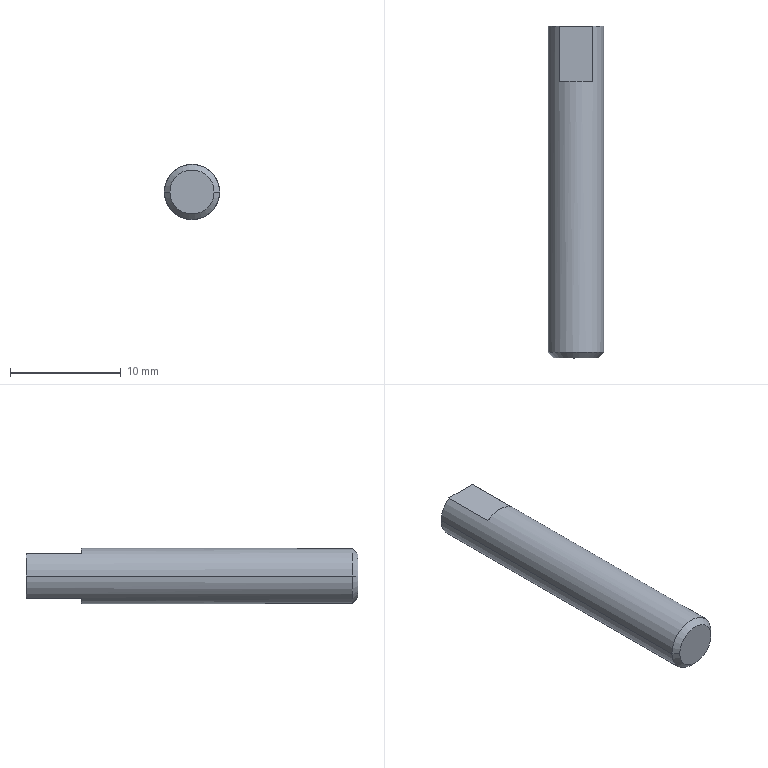Part | STEP file | BU-C08b-2 | 1 solid | 10 faces | box 5 x 30 x 5 mm | volume 576.997 mm3 | plane 6 | cone 2 | cylinder 2 | commonest cylinder face diameters 5 x2
STEP:
#1=CARTESIAN_POINT('',(0.,0.,0.));
#2=DIRECTION('',(0.,0.,1.));
#3=DIRECTION('',(1.,0.,0.));
#4=AXIS2_PLACEMENT_3D('',#1,#2,#3);
#5=CARTESIAN_POINT('',(2.,0.,0.));
#6=VERTEX_POINT('',#5);
#7=CARTESIAN_POINT('',(-2.,0.,0.));
#8=VERTEX_POINT('',#7);
#9=CARTESIAN_POINT('',(0.,0.,0.));
#10=DIRECTION('',(0.,-1.,0.));
#11=DIRECTION('',(1.,0.,0.));
#12=AXIS2_PLACEMENT_3D('',#9,#10,#11);
#13=CIRCLE('',#12,2.);
#14=CARTESIAN_POINT('',(0.,0.,0.));
#15=DIRECTION('',(0.,1.,0.));
#16=DIRECTION('',(-1.,0.,0.));
#17=AXIS2_PLACEMENT_3D('',#14,#15,#16);
#18=CONICAL_SURFACE('',#17,2.,0.7854);
#19=CARTESIAN_POINT('',(3.142,0.));
#20=DIRECTION('',(-1.,0.));
#21=VECTOR('',#20,1.);
#22=LINE('',#19,#21);
#23=(GEOMETRIC_REPRESENTATION_CONTEXT(2)PARAMETRIC_REPRESENTATION_CONTEXT()REPRESENTATION_CONTEXT('',''));
#24=DEFINITIONAL_REPRESENTATION('',(#22),#23);
#25=PCURVE('',#18,#24);
#26=CARTESIAN_POINT('',(0.,0.,0.));
#27=DIRECTION('',(0.,-1.,0.));
#28=DIRECTION('',(1.,0.,0.));
#29=AXIS2_PLACEMENT_3D('',#26,#27,#28);
#30=PLANE('',#29);
#31=CARTESIAN_POINT('',(0.,0.));
#32=DIRECTION('',(1.,0.));
#33=AXIS2_PLACEMENT_2D('',#31,#32);
#34=CIRCLE('',#33,2.);
#35=(GEOMETRIC_REPRESENTATION_CONTEXT(2)PARAMETRIC_REPRESENTATION_CONTEXT()REPRESENTATION_CONTEXT('',''));
#36=DEFINITIONAL_REPRESENTATION('',(#34),#35);
#37=PCURVE('',#30,#36);
#38=SURFACE_CURVE('',#13,(#25,#37),.PCURVE_S1.);
#39=EDGE_CURVE('',#6,#8,#38,.T.);
#40=ORIENTED_EDGE('',*,*,#39,.F.);
#41=CARTESIAN_POINT('',(2.5,0.5,0.));
#42=VERTEX_POINT('',#41);
#43=CARTESIAN_POINT('',(2.,0.,0.));
#44=DIRECTION('',(0.7071,0.7071,0.));
#45=VECTOR('',#44,1.);
#46=LINE('',#43,#45);
#47=CARTESIAN_POINT('',(3.142,0.));
#48=DIRECTION('',(0.,1.));
#49=VECTOR('',#48,1.);
#50=LINE('',#47,#49);
#51=(GEOMETRIC_REPRESENTATION_CONTEXT(2)PARAMETRIC_REPRESENTATION_CONTEXT()REPRESENTATION_CONTEXT('',''));
#52=DEFINITIONAL_REPRESENTATION('',(#50),#51);
#53=PCURVE('',#18,#52);
#54=CARTESIAN_POINT('',(0.,0.,0.));
#55=DIRECTION('',(0.,1.,0.));
#56=DIRECTION('',(-1.,0.,0.));
#57=AXIS2_PLACEMENT_3D('',#54,#55,#56);
#58=CONICAL_SURFACE('',#57,2.,0.7854);
#59=CARTESIAN_POINT('',(3.142,0.));
#60=DIRECTION('',(0.,1.));
#61=VECTOR('',#60,1.);
#62=LINE('',#59,#61);
#63=(GEOMETRIC_REPRESENTATION_CONTEXT(2)PARAMETRIC_REPRESENTATION_CONTEXT()REPRESENTATION_CONTEXT('',''));
#64=DEFINITIONAL_REPRESENTATION('',(#62),#63);
#65=PCURVE('',#58,#64);
#66=SURFACE_CURVE('',#46,(#53,#65),.PCURVE_S1.);
#67=EDGE_CURVE('',#6,#42,#66,.T.);
#68=ORIENTED_EDGE('',*,*,#67,.T.);
#69=CARTESIAN_POINT('',(-2.5,0.5,0.));
#70=VERTEX_POINT('',#69);
#71=CARTESIAN_POINT('',(0.,0.5,0.));
#72=DIRECTION('',(0.,1.,0.));
#73=DIRECTION('',(1.,0.,0.));
#74=AXIS2_PLACEMENT_3D('',#71,#72,#73);
#75=CIRCLE('',#74,2.5);
#76=CARTESIAN_POINT('',(-3.142,0.5));
#77=DIRECTION('',(1.,0.));
#78=VECTOR('',#77,1.);
#79=LINE('',#76,#78);
#80=(GEOMETRIC_REPRESENTATION_CONTEXT(2)PARAMETRIC_REPRESENTATION_CONTEXT()REPRESENTATION_CONTEXT('',''));
#81=DEFINITIONAL_REPRESENTATION('',(#79),#80);
#82=PCURVE('',#18,#81);
#83=CARTESIAN_POINT('',(0.,-1000.,0.));
#84=DIRECTION('',(0.,-1.,0.));
#85=DIRECTION('',(1.,0.,0.));
#86=AXIS2_PLACEMENT_3D('',#83,#84,#85);
#87=CYLINDRICAL_SURFACE('',#86,2.5);
#88=CARTESIAN_POINT('',(6.283,-1000.5));
#89=DIRECTION('',(-1.,0.));
#90=VECTOR('',#89,1.);
#91=LINE('',#88,#90);
#92=(GEOMETRIC_REPRESENTATION_CONTEXT(2)PARAMETRIC_REPRESENTATION_CONTEXT()REPRESENTATION_CONTEXT('',''));
#93=DEFINITIONAL_REPRESENTATION('',(#91),#92);
#94=PCURVE('',#87,#93);
#95=SURFACE_CURVE('',#75,(#82,#94),.PCURVE_S1.);
#96=EDGE_CURVE('',#70,#42,#95,.T.);
#97=ORIENTED_EDGE('',*,*,#96,.F.);
#98=CARTESIAN_POINT('',(-2.,0.,0.));
#99=DIRECTION('',(-0.7071,0.7071,0.));
#100=VECTOR('',#99,1.);
#101=LINE('',#98,#100);
#102=CARTESIAN_POINT('',(0.,0.));
#103=DIRECTION('',(0.,1.));
#104=VECTOR('',#103,1.);
#105=LINE('',#102,#104);
#106=(GEOMETRIC_REPRESENTATION_CONTEXT(2)PARAMETRIC_REPRESENTATION_CONTEXT()REPRESENTATION_CONTEXT('',''));
#107=DEFINITIONAL_REPRESENTATION('',(#105),#106);
#108=PCURVE('',#18,#107);
#109=CARTESIAN_POINT('',(6.283,0.));
#110=DIRECTION('',(0.,1.));
#111=VECTOR('',#110,1.);
#112=LINE('',#109,#111);
#113=(GEOMETRIC_REPRESENTATION_CONTEXT(2)PARAMETRIC_REPRESENTATION_CONTEXT()REPRESENTATION_CONTEXT('',''));
#114=DEFINITIONAL_REPRESENTATION('',(#112),#113);
#115=PCURVE('',#58,#114);
#116=SURFACE_CURVE('',#101,(#108,#115),.PCURVE_S1.);
#117=EDGE_CURVE('',#8,#70,#116,.T.);
#118=ORIENTED_EDGE('',*,*,#117,.F.);
#119=EDGE_LOOP('',(#40,#68,#97,#118));
#120=FACE_BOUND('',#119,.T.);
#121=ADVANCED_FACE('',(#120),#18,.T.);
#122=CARTESIAN_POINT('',(-1.5,30.,2.));
#123=VERTEX_POINT('',#122);
#124=CARTESIAN_POINT('',(-2.5,30.,0.));
#125=VERTEX_POINT('',#124);
#126=CARTESIAN_POINT('',(0.,30.,0.));
#127=DIRECTION('',(0.,-1.,0.));
#128=DIRECTION('',(1.,0.,0.));
#129=AXIS2_PLACEMENT_3D('',#126,#127,#128);
#130=CIRCLE('',#129,2.5);
#131=CARTESIAN_POINT('',(0.,-1030.));
#132=DIRECTION('',(1.,0.));
#133=VECTOR('',#132,1.);
#134=LINE('',#131,#133);
#135=(GEOMETRIC_REPRESENTATION_CONTEXT(2)PARAMETRIC_REPRESENTATION_CONTEXT()REPRESENTATION_CONTEXT('',''));
#136=DEFINITIONAL_REPRESENTATION('',(#134),#135);
#137=PCURVE('',#87,#136);
#138=CARTESIAN_POINT('',(0.,30.,0.));
#139=DIRECTION('',(0.,1.,0.));
#140=DIRECTION('',(-1.,0.,0.));
#141=AXIS2_PLACEMENT_3D('',#138,#139,#140);
#142=PLANE('',#141);
#143=CARTESIAN_POINT('',(-2.5,0.));
#144=CARTESIAN_POINT('',(-2.5,4.33));
#145=CARTESIAN_POINT('',(1.25,2.165));
#146=CARTESIAN_POINT('',(5.,0.));
#147=CARTESIAN_POINT('',(1.25,-2.165));
#148=CARTESIAN_POINT('',(-2.5,-4.33));
#149=CARTESIAN_POINT('',(-2.5,0.));
#150=(BOUNDED_CURVE()B_SPLINE_CURVE(2,(#143,#144,#145,#146,#147,#148,#149),.UNSPECIFIED.,.T.,.F.)B_SPLINE_CURVE_WITH_KNOTS((1,2,2,2,2,1),(-2.094,0.,2.094,4.189,6.283,8.378),.UNSPECIFIED.)CURVE()GEOMETRIC_REPRESENTATION_ITEM()RATIONAL_B_SPLINE_CURVE((1.,0.5,1.,0.5,1.,0.5,1.))REPRESENTATION_ITEM(''));
#151=(GEOMETRIC_REPRESENTATION_CONTEXT(2)PARAMETRIC_REPRESENTATION_CONTEXT()REPRESENTATION_CONTEXT('',''));
#152=DEFINITIONAL_REPRESENTATION('',(#150),#151);
#153=PCURVE('',#142,#152);
#154=SURFACE_CURVE('',#130,(#137,#153),.PCURVE_S1.);
#155=EDGE_CURVE('',#123,#125,#154,.T.);
#156=ORIENTED_EDGE('',*,*,#155,.T.);
#157=CARTESIAN_POINT('',(-2.5,-1000.,0.));
#158=DIRECTION('',(0.,-1.,0.));
#159=VECTOR('',#158,1.);
#160=LINE('',#157,#159);
#161=CARTESIAN_POINT('',(3.142,0.));
#162=DIRECTION('',(0.,1.));
#163=VECTOR('',#162,1.);
#164=LINE('',#161,#163);
#165=(GEOMETRIC_REPRESENTATION_CONTEXT(2)PARAMETRIC_REPRESENTATION_CONTEXT()REPRESENTATION_CONTEXT('',''));
#166=DEFINITIONAL_REPRESENTATION('',(#164),#165);
#167=PCURVE('',#87,#166);
#168=CARTESIAN_POINT('',(0.,-1000.,0.));
#169=DIRECTION('',(0.,-1.,0.));
#170=DIRECTION('',(1.,0.,0.));
#171=AXIS2_PLACEMENT_3D('',#168,#169,#170);
#172=CYLINDRICAL_SURFACE('',#171,2.5);
#173=CARTESIAN_POINT('',(3.142,0.));
#174=DIRECTION('',(0.,1.));
#175=VECTOR('',#174,1.);
#176=LINE('',#173,#175);
#177=(GEOMETRIC_REPRESENTATION_CONTEXT(2)PARAMETRIC_REPRESENTATION_CONTEXT()REPRESENTATION_CONTEXT('',''));
#178=DEFINITIONAL_REPRESENTATION('',(#176),#177);
#179=PCURVE('',#172,#178);
#180=SURFACE_CURVE('',#160,(#167,#179),.PCURVE_S1.);
#181=EDGE_CURVE('',#125,#70,#180,.T.);
#182=ORIENTED_EDGE('',*,*,#181,.T.);
#183=ORIENTED_EDGE('',*,*,#96,.T.);
#184=CARTESIAN_POINT('',(2.5,30.,0.));
#185=VERTEX_POINT('',#184);
#186=CARTESIAN_POINT('',(2.5,-1000.,0.));
#187=DIRECTION('',(0.,-1.,0.));
#188=VECTOR('',#187,1.);
#189=LINE('',#186,#188);
#190=CARTESIAN_POINT('',(0.,0.));
#191=DIRECTION('',(0.,1.));
#192=VECTOR('',#191,1.);
#193=LINE('',#190,#192);
#194=(GEOMETRIC_REPRESENTATION_CONTEXT(2)PARAMETRIC_REPRESENTATION_CONTEXT()REPRESENTATION_CONTEXT('',''));
#195=DEFINITIONAL_REPRESENTATION('',(#193),#194);
#196=PCURVE('',#87,#195);
#197=CARTESIAN_POINT('',(6.283,0.));
#198=DIRECTION('',(0.,1.));
#199=VECTOR('',#198,1.);
#200=LINE('',#197,#199);
#201=(GEOMETRIC_REPRESENTATION_CONTEXT(2)PARAMETRIC_REPRESENTATION_CONTEXT()REPRESENTATION_CONTEXT('',''));
#202=DEFINITIONAL_REPRESENTATION('',(#200),#201);
#203=PCURVE('',#172,#202);
#204=SURFACE_CURVE('',#189,(#196,#203),.PCURVE_S1.);
#205=EDGE_CURVE('',#185,#42,#204,.T.);
#206=ORIENTED_EDGE('',*,*,#205,.F.);
#207=CARTESIAN_POINT('',(1.5,30.,2.));
#208=VERTEX_POINT('',#207);
#209=CARTESIAN_POINT('',(0.,30.,0.));
#210=DIRECTION('',(0.,-1.,0.));
#211=DIRECTION('',(1.,0.,0.));
#212=AXIS2_PLACEMENT_3D('',#209,#210,#211);
#213=CIRCLE('',#212,2.5);
#214=CARTESIAN_POINT('',(0.,-1030.));
#215=DIRECTION('',(1.,0.));
#216=VECTOR('',#215,1.);
#217=LINE('',#214,#216);
#218=(GEOMETRIC_REPRESENTATION_CONTEXT(2)PARAMETRIC_REPRESENTATION_CONTEXT()REPRESENTATION_CONTEXT('',''));
#219=DEFINITIONAL_REPRESENTATION('',(#217),#218);
#220=PCURVE('',#87,#219);
#221=CARTESIAN_POINT('',(-2.5,0.));
#222=CARTESIAN_POINT('',(-2.5,4.33));
#223=CARTESIAN_POINT('',(1.25,2.165));
#224=CARTESIAN_POINT('',(5.,0.));
#225=CARTESIAN_POINT('',(1.25,-2.165));
#226=CARTESIAN_POINT('',(-2.5,-4.33));
#227=CARTESIAN_POINT('',(-2.5,0.));
#228=(BOUNDED_CURVE()B_SPLINE_CURVE(2,(#221,#222,#223,#224,#225,#226,#227),.UNSPECIFIED.,.T.,.F.)B_SPLINE_CURVE_WITH_KNOTS((1,2,2,2,2,1),(-2.094,0.,2.094,4.189,6.283,8.378),.UNSPECIFIED.)CURVE()GEOMETRIC_REPRESENTATION_ITEM()RATIONAL_B_SPLINE_CURVE((1.,0.5,1.,0.5,1.,0.5,1.))REPRESENTATION_ITEM(''));
#229=(GEOMETRIC_REPRESENTATION_CONTEXT(2)PARAMETRIC_REPRESENTATION_CONTEXT()REPRESENTATION_CONTEXT('',''));
#230=DEFINITIONAL_REPRESENTATION('',(#228),#229);
#231=PCURVE('',#142,#230);
#232=SURFACE_CURVE('',#213,(#220,#231),.PCURVE_S1.);
#233=EDGE_CURVE('',#185,#208,#232,.T.);
#234=ORIENTED_EDGE('',*,*,#233,.T.);
#235=CARTESIAN_POINT('',(1.5,25.,2.));
#236=VERTEX_POINT('',#235);
#237=CARTESIAN_POINT('',(1.5,25.,2.));
#238=DIRECTION('',(0.,1.,0.));
#239=VECTOR('',#238,1.);
#240=LINE('',#237,#239);
#241=CARTESIAN_POINT('',(0.9273,-1025.));
#242=DIRECTION('',(0.,-1.));
#243=VECTOR('',#242,1.);
#244=LINE('',#241,#243);
#245=(GEOMETRIC_REPRESENTATION_CONTEXT(2)PARAMETRIC_REPRESENTATION_CONTEXT()REPRESENTATION_CONTEXT('',''));
#246=DEFINITIONAL_REPRESENTATION('',(#244),#245);
#247=PCURVE('',#87,#246);
#248=CARTESIAN_POINT('',(-1.5,25.,2.));
#249=DIRECTION('',(0.,0.,-1.));
#250=DIRECTION('',(-1.,0.,0.));
#251=AXIS2_PLACEMENT_3D('',#248,#249,#250);
#252=PLANE('',#251);
#253=CARTESIAN_POINT('',(-3.,0.));
#254=DIRECTION('',(0.,1.));
#255=VECTOR('',#254,1.);
#256=LINE('',#253,#255);
#257=(GEOMETRIC_REPRESENTATION_CONTEXT(2)PARAMETRIC_REPRESENTATION_CONTEXT()REPRESENTATION_CONTEXT('',''));
#258=DEFINITIONAL_REPRESENTATION('',(#256),#257);
#259=PCURVE('',#252,#258);
#260=SURFACE_CURVE('',#240,(#247,#259),.PCURVE_S1.);
#261=EDGE_CURVE('',#236,#208,#260,.T.);
#262=ORIENTED_EDGE('',*,*,#261,.F.);
#263=CARTESIAN_POINT('',(-1.5,25.,2.));
#264=VERTEX_POINT('',#263);
#265=CARTESIAN_POINT('',(0.,25.,0.));
#266=DIRECTION('',(0.,1.,0.));
#267=DIRECTION('',(-1.,0.,0.));
#268=AXIS2_PLACEMENT_3D('',#265,#266,#267);
#269=CIRCLE('',#268,2.5);
#270=CARTESIAN_POINT('',(3.142,-1025.));
#271=DIRECTION('',(-1.,0.));
#272=VECTOR('',#271,1.);
#273=LINE('',#270,#272);
#274=(GEOMETRIC_REPRESENTATION_CONTEXT(2)PARAMETRIC_REPRESENTATION_CONTEXT()REPRESENTATION_CONTEXT('',''));
#275=DEFINITIONAL_REPRESENTATION('',(#273),#274);
#276=PCURVE('',#87,#275);
#277=CARTESIAN_POINT('',(0.,25.,0.));
#278=DIRECTION('',(0.,1.,0.));
#279=DIRECTION('',(-1.,0.,0.));
#280=AXIS2_PLACEMENT_3D('',#277,#278,#279);
#281=PLANE('',#280);
#282=CARTESIAN_POINT('',(0.,0.));
#283=DIRECTION('',(1.,0.));
#284=AXIS2_PLACEMENT_2D('',#282,#283);
#285=CIRCLE('',#284,2.5);
#286=(GEOMETRIC_REPRESENTATION_CONTEXT(2)PARAMETRIC_REPRESENTATION_CONTEXT()REPRESENTATION_CONTEXT('',''));
#287=DEFINITIONAL_REPRESENTATION('',(#285),#286);
#288=PCURVE('',#281,#287);
#289=SURFACE_CURVE('',#269,(#276,#288),.PCURVE_S1.);
#290=EDGE_CURVE('',#264,#236,#289,.T.);
#291=ORIENTED_EDGE('',*,*,#290,.F.);
#292=CARTESIAN_POINT('',(-1.5,25.,2.));
#293=DIRECTION('',(0.,1.,0.));
#294=VECTOR('',#293,1.);
#295=LINE('',#292,#294);
#296=CARTESIAN_POINT('',(2.214,-1025.));
#297=DIRECTION('',(0.,-1.));
#298=VECTOR('',#297,1.);
#299=LINE('',#296,#298);
#300=(GEOMETRIC_REPRESENTATION_CONTEXT(2)PARAMETRIC_REPRESENTATION_CONTEXT()REPRESENTATION_CONTEXT('',''));
#301=DEFINITIONAL_REPRESENTATION('',(#299),#300);
#302=PCURVE('',#87,#301);
#303=CARTESIAN_POINT('',(0.,0.));
#304=DIRECTION('',(0.,1.));
#305=VECTOR('',#304,1.);
#306=LINE('',#303,#305);
#307=(GEOMETRIC_REPRESENTATION_CONTEXT(2)PARAMETRIC_REPRESENTATION_CONTEXT()REPRESENTATION_CONTEXT('',''));
#308=DEFINITIONAL_REPRESENTATION('',(#306),#307);
#309=PCURVE('',#252,#308);
#310=SURFACE_CURVE('',#295,(#302,#309),.PCURVE_S1.);
#311=EDGE_CURVE('',#264,#123,#310,.T.);
#312=ORIENTED_EDGE('',*,*,#311,.T.);
#313=EDGE_LOOP('',(#156,#182,#183,#206,#234,#262,#291,#312));
#314=FACE_BOUND('',#313,.T.);
#315=ADVANCED_FACE('',(#314),#87,.T.);
#316=CARTESIAN_POINT('',(-1.5,30.,2.));
#317=DIRECTION('',(-1.,0.,0.));
#318=VECTOR('',#317,1.);
#319=LINE('',#316,#318);
#320=CARTESIAN_POINT('',(1.5,2.));
#321=DIRECTION('',(1.,0.));
#322=VECTOR('',#321,1.);
#323=LINE('',#320,#322);
#324=(GEOMETRIC_REPRESENTATION_CONTEXT(2)PARAMETRIC_REPRESENTATION_CONTEXT()REPRESENTATION_CONTEXT('',''));
#325=DEFINITIONAL_REPRESENTATION('',(#323),#324);
#326=PCURVE('',#142,#325);
#327=CARTESIAN_POINT('',(0.,5.));
#328=DIRECTION('',(1.,0.));
#329=VECTOR('',#328,1.);
#330=LINE('',#327,#329);
#331=(GEOMETRIC_REPRESENTATION_CONTEXT(2)PARAMETRIC_REPRESENTATION_CONTEXT()REPRESENTATION_CONTEXT('',''));
#332=DEFINITIONAL_REPRESENTATION('',(#330),#331);
#333=PCURVE('',#252,#332);
#334=SURFACE_CURVE('',#319,(#326,#333),.PCURVE_S1.);
#335=EDGE_CURVE('',#208,#123,#334,.T.);
#336=ORIENTED_EDGE('',*,*,#335,.F.);
#337=ORIENTED_EDGE('',*,*,#233,.F.);
#338=CARTESIAN_POINT('',(1.5,30.,-2.));
#339=VERTEX_POINT('',#338);
#340=CARTESIAN_POINT('',(0.,30.,0.));
#341=DIRECTION('',(0.,-1.,0.));
#342=DIRECTION('',(1.,0.,0.));
#343=AXIS2_PLACEMENT_3D('',#340,#341,#342);
#344=CIRCLE('',#343,2.5);
#345=CARTESIAN_POINT('',(-2.5,0.));
#346=CARTESIAN_POINT('',(-2.5,4.33));
#347=CARTESIAN_POINT('',(1.25,2.165));
#348=CARTESIAN_POINT('',(5.,0.));
#349=CARTESIAN_POINT('',(1.25,-2.165));
#350=CARTESIAN_POINT('',(-2.5,-4.33));
#351=CARTESIAN_POINT('',(-2.5,0.));
#352=(BOUNDED_CURVE()B_SPLINE_CURVE(2,(#345,#346,#347,#348,#349,#350,#351),.UNSPECIFIED.,.T.,.F.)B_SPLINE_CURVE_WITH_KNOTS((1,2,2,2,2,1),(-2.094,0.,2.094,4.189,6.283,8.378),.UNSPECIFIED.)CURVE()GEOMETRIC_REPRESENTATION_ITEM()RATIONAL_B_SPLINE_CURVE((1.,0.5,1.,0.5,1.,0.5,1.))REPRESENTATION_ITEM(''));
#353=(GEOMETRIC_REPRESENTATION_CONTEXT(2)PARAMETRIC_REPRESENTATION_CONTEXT()REPRESENTATION_CONTEXT('',''));
#354=DEFINITIONAL_REPRESENTATION('',(#352),#353);
#355=PCURVE('',#142,#354);
#356=CARTESIAN_POINT('',(0.,-1030.));
#357=DIRECTION('',(1.,0.));
#358=VECTOR('',#357,1.);
#359=LINE('',#356,#358);
#360=(GEOMETRIC_REPRESENTATION_CONTEXT(2)PARAMETRIC_REPRESENTATION_CONTEXT()REPRESENTATION_CONTEXT('',''));
#361=DEFINITIONAL_REPRESENTATION('',(#359),#360);
#362=PCURVE('',#172,#361);
#363=SURFACE_CURVE('',#344,(#355,#362),.PCURVE_S1.);
#364=EDGE_CURVE('',#339,#185,#363,.T.);
#365=ORIENTED_EDGE('',*,*,#364,.F.);
#366=CARTESIAN_POINT('',(-1.5,30.,-2.));
#367=VERTEX_POINT('',#366);
#368=CARTESIAN_POINT('',(-1.5,30.,-2.));
#369=DIRECTION('',(1.,0.,0.));
#370=VECTOR('',#369,1.);
#371=LINE('',#368,#370);
#372=CARTESIAN_POINT('',(1.5,-2.));
#373=DIRECTION('',(-1.,0.));
#374=VECTOR('',#373,1.);
#375=LINE('',#372,#374);
#376=(GEOMETRIC_REPRESENTATION_CONTEXT(2)PARAMETRIC_REPRESENTATION_CONTEXT()REPRESENTATION_CONTEXT('',''));
#377=DEFINITIONAL_REPRESENTATION('',(#375),#376);
#378=PCURVE('',#142,#377);
#379=CARTESIAN_POINT('',(-1.5,25.,-2.));
#380=DIRECTION('',(0.,0.,1.));
#381=DIRECTION('',(1.,0.,0.));
#382=AXIS2_PLACEMENT_3D('',#379,#380,#381);
#383=PLANE('',#382);
#384=CARTESIAN_POINT('',(0.,5.));
#385=DIRECTION('',(1.,0.));
#386=VECTOR('',#385,1.);
#387=LINE('',#384,#386);
#388=(GEOMETRIC_REPRESENTATION_CONTEXT(2)PARAMETRIC_REPRESENTATION_CONTEXT()REPRESENTATION_CONTEXT('',''));
#389=DEFINITIONAL_REPRESENTATION('',(#387),#388);
#390=PCURVE('',#383,#389);
#391=SURFACE_CURVE('',#371,(#378,#390),.PCURVE_S1.);
#392=EDGE_CURVE('',#367,#339,#391,.T.);
#393=ORIENTED_EDGE('',*,*,#392,.F.);
#394=CARTESIAN_POINT('',(0.,30.,0.));
#395=DIRECTION('',(0.,-1.,0.));
#396=DIRECTION('',(1.,0.,0.));
#397=AXIS2_PLACEMENT_3D('',#394,#395,#396);
#398=CIRCLE('',#397,2.5);
#399=CARTESIAN_POINT('',(-2.5,0.));
#400=CARTESIAN_POINT('',(-2.5,4.33));
#401=CARTESIAN_POINT('',(1.25,2.165));
#402=CARTESIAN_POINT('',(5.,0.));
#403=CARTESIAN_POINT('',(1.25,-2.165));
#404=CARTESIAN_POINT('',(-2.5,-4.33));
#405=CARTESIAN_POINT('',(-2.5,0.));
#406=(BOUNDED_CURVE()B_SPLINE_CURVE(2,(#399,#400,#401,#402,#403,#404,#405),.UNSPECIFIED.,.T.,.F.)B_SPLINE_CURVE_WITH_KNOTS((1,2,2,2,2,1),(-2.094,0.,2.094,4.189,6.283,8.378),.UNSPECIFIED.)CURVE()GEOMETRIC_REPRESENTATION_ITEM()RATIONAL_B_SPLINE_CURVE((1.,0.5,1.,0.5,1.,0.5,1.))REPRESENTATION_ITEM(''));
#407=(GEOMETRIC_REPRESENTATION_CONTEXT(2)PARAMETRIC_REPRESENTATION_CONTEXT()REPRESENTATION_CONTEXT('',''));
#408=DEFINITIONAL_REPRESENTATION('',(#406),#407);
#409=PCURVE('',#142,#408);
#410=CARTESIAN_POINT('',(0.,-1030.));
#411=DIRECTION('',(1.,0.));
#412=VECTOR('',#411,1.);
#413=LINE('',#410,#412);
#414=(GEOMETRIC_REPRESENTATION_CONTEXT(2)PARAMETRIC_REPRESENTATION_CONTEXT()REPRESENTATION_CONTEXT('',''));
#415=DEFINITIONAL_REPRESENTATION('',(#413),#414);
#416=PCURVE('',#172,#415);
#417=SURFACE_CURVE('',#398,(#409,#416),.PCURVE_S1.);
#418=EDGE_CURVE('',#125,#367,#417,.T.);
#419=ORIENTED_EDGE('',*,*,#418,.F.);
#420=ORIENTED_EDGE('',*,*,#155,.F.);
#421=EDGE_LOOP('',(#336,#337,#365,#393,#419,#420));
#422=FACE_BOUND('',#421,.T.);
#423=ADVANCED_FACE('',(#422),#142,.T.);
#424=ORIENTED_EDGE('',*,*,#181,.F.);
#425=ORIENTED_EDGE('',*,*,#418,.T.);
#426=CARTESIAN_POINT('',(-1.5,25.,-2.));
#427=VERTEX_POINT('',#426);
#428=CARTESIAN_POINT('',(-1.5,25.,-2.));
#429=DIRECTION('',(0.,1.,0.));
#430=VECTOR('',#429,1.);
#431=LINE('',#428,#430);
#432=CARTESIAN_POINT('',(4.069,-1025.));
#433=DIRECTION('',(0.,-1.));
#434=VECTOR('',#433,1.);
#435=LINE('',#432,#434);
#436=(GEOMETRIC_REPRESENTATION_CONTEXT(2)PARAMETRIC_REPRESENTATION_CONTEXT()REPRESENTATION_CONTEXT('',''));
#437=DEFINITIONAL_REPRESENTATION('',(#435),#436);
#438=PCURVE('',#172,#437);
#439=CARTESIAN_POINT('',(0.,0.));
#440=DIRECTION('',(0.,1.));
#441=VECTOR('',#440,1.);
#442=LINE('',#439,#441);
#443=(GEOMETRIC_REPRESENTATION_CONTEXT(2)PARAMETRIC_REPRESENTATION_CONTEXT()REPRESENTATION_CONTEXT('',''));
#444=DEFINITIONAL_REPRESENTATION('',(#442),#443);
#445=PCURVE('',#383,#444);
#446=SURFACE_CURVE('',#431,(#438,#445),.PCURVE_S1.);
#447=EDGE_CURVE('',#427,#367,#446,.T.);
#448=ORIENTED_EDGE('',*,*,#447,.F.);
#449=CARTESIAN_POINT('',(1.5,25.,-2.));
#450=VERTEX_POINT('',#449);
#451=CARTESIAN_POINT('',(0.,25.,0.));
#452=DIRECTION('',(0.,1.,0.));
#453=DIRECTION('',(-1.,0.,0.));
#454=AXIS2_PLACEMENT_3D('',#451,#452,#453);
#455=CIRCLE('',#454,2.5);
#456=CARTESIAN_POINT('',(9.425,-1025.));
#457=DIRECTION('',(-1.,0.));
#458=VECTOR('',#457,1.);
#459=LINE('',#456,#458);
#460=(GEOMETRIC_REPRESENTATION_CONTEXT(2)PARAMETRIC_REPRESENTATION_CONTEXT()REPRESENTATION_CONTEXT('',''));
#461=DEFINITIONAL_REPRESENTATION('',(#459),#460);
#462=PCURVE('',#172,#461);
#463=CARTESIAN_POINT('',(0.,25.,0.));
#464=DIRECTION('',(0.,1.,0.));
#465=DIRECTION('',(-1.,0.,0.));
#466=AXIS2_PLACEMENT_3D('',#463,#464,#465);
#467=PLANE('',#466);
#468=CARTESIAN_POINT('',(0.,0.));
#469=DIRECTION('',(1.,0.));
#470=AXIS2_PLACEMENT_2D('',#468,#469);
#471=CIRCLE('',#470,2.5);
#472=(GEOMETRIC_REPRESENTATION_CONTEXT(2)PARAMETRIC_REPRESENTATION_CONTEXT()REPRESENTATION_CONTEXT('',''));
#473=DEFINITIONAL_REPRESENTATION('',(#471),#472);
#474=PCURVE('',#467,#473);
#475=SURFACE_CURVE('',#455,(#462,#474),.PCURVE_S1.);
#476=EDGE_CURVE('',#450,#427,#475,.T.);
#477=ORIENTED_EDGE('',*,*,#476,.F.);
#478=CARTESIAN_POINT('',(1.5,25.,-2.));
#479=DIRECTION('',(0.,1.,0.));
#480=VECTOR('',#479,1.);
#481=LINE('',#478,#480);
#482=CARTESIAN_POINT('',(5.356,-1025.));
#483=DIRECTION('',(0.,-1.));
#484=VECTOR('',#483,1.);
#485=LINE('',#482,#484);
#486=(GEOMETRIC_REPRESENTATION_CONTEXT(2)PARAMETRIC_REPRESENTATION_CONTEXT()REPRESENTATION_CONTEXT('',''));
#487=DEFINITIONAL_REPRESENTATION('',(#485),#486);
#488=PCURVE('',#172,#487);
#489=CARTESIAN_POINT('',(3.,0.));
#490=DIRECTION('',(0.,1.));
#491=VECTOR('',#490,1.);
#492=LINE('',#489,#491);
#493=(GEOMETRIC_REPRESENTATION_CONTEXT(2)PARAMETRIC_REPRESENTATION_CONTEXT()REPRESENTATION_CONTEXT('',''));
#494=DEFINITIONAL_REPRESENTATION('',(#492),#493);
#495=PCURVE('',#383,#494);
#496=SURFACE_CURVE('',#481,(#488,#495),.PCURVE_S1.);
#497=EDGE_CURVE('',#450,#339,#496,.T.);
#498=ORIENTED_EDGE('',*,*,#497,.T.);
#499=ORIENTED_EDGE('',*,*,#364,.T.);
#500=ORIENTED_EDGE('',*,*,#205,.T.);
#501=CARTESIAN_POINT('',(0.,0.5,0.));
#502=DIRECTION('',(0.,1.,0.));
#503=DIRECTION('',(1.,0.,0.));
#504=AXIS2_PLACEMENT_3D('',#501,#502,#503);
#505=CIRCLE('',#504,2.5);
#506=CARTESIAN_POINT('',(6.283,-1000.5));
#507=DIRECTION('',(-1.,0.));
#508=VECTOR('',#507,1.);
#509=LINE('',#506,#508);
#510=(GEOMETRIC_REPRESENTATION_CONTEXT(2)PARAMETRIC_REPRESENTATION_CONTEXT()REPRESENTATION_CONTEXT('',''));
#511=DEFINITIONAL_REPRESENTATION('',(#509),#510);
#512=PCURVE('',#172,#511);
#513=CARTESIAN_POINT('',(3.142,0.5));
#514=DIRECTION('',(1.,0.));
#515=VECTOR('',#514,1.);
#516=LINE('',#513,#515);
#517=(GEOMETRIC_REPRESENTATION_CONTEXT(2)PARAMETRIC_REPRESENTATION_CONTEXT()REPRESENTATION_CONTEXT('',''));
#518=DEFINITIONAL_REPRESENTATION('',(#516),#517);
#519=PCURVE('',#58,#518);
#520=SURFACE_CURVE('',#505,(#512,#519),.PCURVE_S1.);
#521=EDGE_CURVE('',#42,#70,#520,.T.);
#522=ORIENTED_EDGE('',*,*,#521,.T.);
#523=EDGE_LOOP('',(#424,#425,#448,#477,#498,#499,#500,#522));
#524=FACE_BOUND('',#523,.T.);
#525=ADVANCED_FACE('',(#524),#172,.T.);
#526=CARTESIAN_POINT('',(0.,0.,0.));
#527=DIRECTION('',(0.,-1.,0.));
#528=DIRECTION('',(1.,0.,0.));
#529=AXIS2_PLACEMENT_3D('',#526,#527,#528);
#530=CIRCLE('',#529,2.);
#531=CARTESIAN_POINT('',(0.,0.));
#532=DIRECTION('',(1.,0.));
#533=AXIS2_PLACEMENT_2D('',#531,#532);
#534=CIRCLE('',#533,2.);
#535=(GEOMETRIC_REPRESENTATION_CONTEXT(2)PARAMETRIC_REPRESENTATION_CONTEXT()REPRESENTATION_CONTEXT('',''));
#536=DEFINITIONAL_REPRESENTATION('',(#534),#535);
#537=PCURVE('',#30,#536);
#538=CARTESIAN_POINT('',(9.425,0.));
#539=DIRECTION('',(-1.,0.));
#540=VECTOR('',#539,1.);
#541=LINE('',#538,#540);
#542=(GEOMETRIC_REPRESENTATION_CONTEXT(2)PARAMETRIC_REPRESENTATION_CONTEXT()REPRESENTATION_CONTEXT('',''));
#543=DEFINITIONAL_REPRESENTATION('',(#541),#542);
#544=PCURVE('',#58,#543);
#545=SURFACE_CURVE('',#530,(#537,#544),.PCURVE_S1.);
#546=EDGE_CURVE('',#8,#6,#545,.T.);
#547=ORIENTED_EDGE('',*,*,#546,.T.);
#548=ORIENTED_EDGE('',*,*,#39,.T.);
#549=EDGE_LOOP('',(#547,#548));
#550=FACE_BOUND('',#549,.T.);
#551=ADVANCED_FACE('',(#550),#30,.T.);
#552=ORIENTED_EDGE('',*,*,#392,.T.);
#553=ORIENTED_EDGE('',*,*,#497,.F.);
#554=CARTESIAN_POINT('',(-1.5,25.,-2.));
#555=DIRECTION('',(1.,0.,0.));
#556=VECTOR('',#555,1.);
#557=LINE('',#554,#556);
#558=CARTESIAN_POINT('',(0.,0.));
#559=DIRECTION('',(1.,0.));
#560=VECTOR('',#559,1.);
#561=LINE('',#558,#560);
#562=(GEOMETRIC_REPRESENTATION_CONTEXT(2)PARAMETRIC_REPRESENTATION_CONTEXT()REPRESENTATION_CONTEXT('',''));
#563=DEFINITIONAL_REPRESENTATION('',(#561),#562);
#564=PCURVE('',#383,#563);
#565=CARTESIAN_POINT('',(1.5,-2.));
#566=DIRECTION('',(-1.,0.));
#567=VECTOR('',#566,1.);
#568=LINE('',#565,#567);
#569=(GEOMETRIC_REPRESENTATION_CONTEXT(2)PARAMETRIC_REPRESENTATION_CONTEXT()REPRESENTATION_CONTEXT('',''));
#570=DEFINITIONAL_REPRESENTATION('',(#568),#569);
#571=PCURVE('',#467,#570);
#572=SURFACE_CURVE('',#557,(#564,#571),.PCURVE_S1.);
#573=EDGE_CURVE('',#427,#450,#572,.T.);
#574=ORIENTED_EDGE('',*,*,#573,.F.);
#575=ORIENTED_EDGE('',*,*,#447,.T.);
#576=EDGE_LOOP('',(#552,#553,#574,#575));
#577=FACE_BOUND('',#576,.T.);
#578=ADVANCED_FACE('',(#577),#383,.F.);
#579=ORIENTED_EDGE('',*,*,#476,.T.);
#580=ORIENTED_EDGE('',*,*,#573,.T.);
#581=EDGE_LOOP('',(#579,#580));
#582=FACE_BOUND('',#581,.T.);
#583=ADVANCED_FACE('',(#582),#467,.T.);
#584=ORIENTED_EDGE('',*,*,#335,.T.);
#585=ORIENTED_EDGE('',*,*,#311,.F.);
#586=CARTESIAN_POINT('',(-1.5,25.,2.));
#587=DIRECTION('',(-1.,0.,0.));
#588=VECTOR('',#587,1.);
#589=LINE('',#586,#588);
#590=CARTESIAN_POINT('',(0.,0.));
#591=DIRECTION('',(1.,0.));
#592=VECTOR('',#591,1.);
#593=LINE('',#590,#592);
#594=(GEOMETRIC_REPRESENTATION_CONTEXT(2)PARAMETRIC_REPRESENTATION_CONTEXT()REPRESENTATION_CONTEXT('',''));
#595=DEFINITIONAL_REPRESENTATION('',(#593),#594);
#596=PCURVE('',#252,#595);
#597=CARTESIAN_POINT('',(1.5,2.));
#598=DIRECTION('',(1.,0.));
#599=VECTOR('',#598,1.);
#600=LINE('',#597,#599);
#601=(GEOMETRIC_REPRESENTATION_CONTEXT(2)PARAMETRIC_REPRESENTATION_CONTEXT()REPRESENTATION_CONTEXT('',''));
#602=DEFINITIONAL_REPRESENTATION('',(#600),#601);
#603=PCURVE('',#281,#602);
#604=SURFACE_CURVE('',#589,(#596,#603),.PCURVE_S1.);
#605=EDGE_CURVE('',#236,#264,#604,.T.);
#606=ORIENTED_EDGE('',*,*,#605,.F.);
#607=ORIENTED_EDGE('',*,*,#261,.T.);
#608=EDGE_LOOP('',(#584,#585,#606,#607));
#609=FACE_BOUND('',#608,.T.);
#610=ADVANCED_FACE('',(#609),#252,.F.);
#611=ORIENTED_EDGE('',*,*,#290,.T.);
#612=ORIENTED_EDGE('',*,*,#605,.T.);
#613=EDGE_LOOP('',(#611,#612));
#614=FACE_BOUND('',#613,.T.);
#615=ADVANCED_FACE('',(#614),#281,.T.);
#616=ORIENTED_EDGE('',*,*,#67,.F.);
#617=ORIENTED_EDGE('',*,*,#546,.F.);
#618=ORIENTED_EDGE('',*,*,#117,.T.);
#619=ORIENTED_EDGE('',*,*,#521,.F.);
#620=EDGE_LOOP('',(#616,#617,#618,#619));
#621=FACE_BOUND('',#620,.T.);
#622=ADVANCED_FACE('',(#621),#58,.T.);
#623=CLOSED_SHELL('',(#121,#315,#423,#525,#551,#578,#583,#610,#615,#622));
#624=MANIFOLD_SOLID_BREP('',#623);
#625=(LENGTH_UNIT()NAMED_UNIT(*)SI_UNIT(.MILLI.,.METRE.));
#626=UNCERTAINTY_MEASURE_WITH_UNIT(LENGTH_MEASURE(0.0000001),#625,'','');
#627=(NAMED_UNIT(*)PLANE_ANGLE_UNIT()SI_UNIT($,.RADIAN.));
#628=(NAMED_UNIT(*)SI_UNIT($,.STERADIAN.)SOLID_ANGLE_UNIT());
#629=(GEOMETRIC_REPRESENTATION_CONTEXT(3)GLOBAL_UNCERTAINTY_ASSIGNED_CONTEXT((#626))GLOBAL_UNIT_ASSIGNED_CONTEXT((#625,#627,#628))REPRESENTATION_CONTEXT('',''));
#630=ADVANCED_BREP_SHAPE_REPRESENTATION('',(#4,#624),#629);